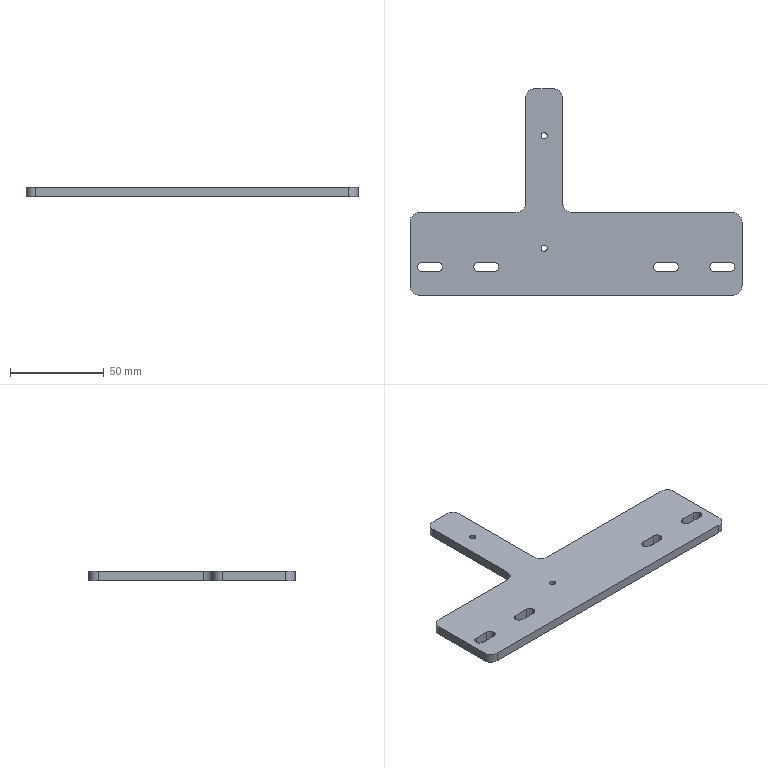Part | 1 solid | 42 faces | box 177 x 110 x 5 mm | volume 44090 mm3 | cylinder 24 | plane 18 | commonest cylinder face diameters 5.2 x12 10 x8 3.3 x4
STEP:
#1=CARTESIAN_POINT('',(-74.3,-40.,0.));
#2=VERTEX_POINT('',#1);
#3=CARTESIAN_POINT('',(-76.9,-37.4,0.));
#4=VERTEX_POINT('',#3);
#5=CARTESIAN_POINT('',(-76.9,-40.,0.));
#6=DIRECTION('',(0.,0.,1.));
#7=DIRECTION('',(1.,0.,0.));
#8=AXIS2_PLACEMENT_3D('',#5,#6,#7);
#9=CIRCLE('',#8,2.6);
#10=EDGE_CURVE('',#2,#4,#9,.T.);
#11=ORIENTED_EDGE('',*,*,#10,.F.);
#12=CARTESIAN_POINT('',(-74.3,-40.,5.));
#13=VERTEX_POINT('',#12);
#14=CARTESIAN_POINT('',(-74.3,-40.,0.));
#15=DIRECTION('',(0.,0.,1.));
#16=VECTOR('',#15,1000.);
#17=LINE('',#14,#16);
#18=EDGE_CURVE('',#2,#13,#17,.T.);
#19=ORIENTED_EDGE('',*,*,#18,.T.);
#20=CARTESIAN_POINT('',(-76.9,-37.4,5.));
#21=VERTEX_POINT('',#20);
#22=CARTESIAN_POINT('',(-76.9,-40.,5.));
#23=DIRECTION('',(0.,0.,1.));
#24=DIRECTION('',(1.,0.,0.));
#25=AXIS2_PLACEMENT_3D('',#22,#23,#24);
#26=CIRCLE('',#25,2.6);
#27=EDGE_CURVE('',#13,#21,#26,.T.);
#28=ORIENTED_EDGE('',*,*,#27,.T.);
#29=CARTESIAN_POINT('',(-76.9,-37.4,0.));
#30=DIRECTION('',(0.,0.,1.));
#31=VECTOR('',#30,1000.);
#32=LINE('',#29,#31);
#33=EDGE_CURVE('',#4,#21,#32,.T.);
#34=ORIENTED_EDGE('',*,*,#33,.F.);
#35=EDGE_LOOP('',(#11,#19,#28,#34));
#36=FACE_OUTER_BOUND('',#35,.T.);
#37=CARTESIAN_POINT('',(-76.9,-40.,0.));
#38=DIRECTION('',(0.,0.,1.));
#39=DIRECTION('',(1.,0.,0.));
#40=AXIS2_PLACEMENT_3D('',#37,#38,#39);
#41=CYLINDRICAL_SURFACE('',#40,2.6);
#42=ADVANCED_FACE('',(#36),#41,.F.);
#43=CARTESIAN_POINT('',(-44.3,-40.,0.));
#44=VERTEX_POINT('',#43);
#45=CARTESIAN_POINT('',(-46.9,-37.4,0.));
#46=VERTEX_POINT('',#45);
#47=CARTESIAN_POINT('',(-46.9,-40.,0.));
#48=DIRECTION('',(0.,0.,1.));
#49=DIRECTION('',(1.,0.,0.));
#50=AXIS2_PLACEMENT_3D('',#47,#48,#49);
#51=CIRCLE('',#50,2.6);
#52=EDGE_CURVE('',#44,#46,#51,.T.);
#53=ORIENTED_EDGE('',*,*,#52,.F.);
#54=CARTESIAN_POINT('',(-44.3,-40.,5.));
#55=VERTEX_POINT('',#54);
#56=CARTESIAN_POINT('',(-44.3,-40.,0.));
#57=DIRECTION('',(0.,0.,1.));
#58=VECTOR('',#57,1000.);
#59=LINE('',#56,#58);
#60=EDGE_CURVE('',#44,#55,#59,.T.);
#61=ORIENTED_EDGE('',*,*,#60,.T.);
#62=CARTESIAN_POINT('',(-46.9,-37.4,5.));
#63=VERTEX_POINT('',#62);
#64=CARTESIAN_POINT('',(-46.9,-40.,5.));
#65=DIRECTION('',(0.,0.,1.));
#66=DIRECTION('',(1.,0.,0.));
#67=AXIS2_PLACEMENT_3D('',#64,#65,#66);
#68=CIRCLE('',#67,2.6);
#69=EDGE_CURVE('',#55,#63,#68,.T.);
#70=ORIENTED_EDGE('',*,*,#69,.T.);
#71=CARTESIAN_POINT('',(-46.9,-37.4,0.));
#72=DIRECTION('',(0.,0.,1.));
#73=VECTOR('',#72,1000.);
#74=LINE('',#71,#73);
#75=EDGE_CURVE('',#46,#63,#74,.T.);
#76=ORIENTED_EDGE('',*,*,#75,.F.);
#77=EDGE_LOOP('',(#53,#61,#70,#76));
#78=FACE_OUTER_BOUND('',#77,.T.);
#79=CARTESIAN_POINT('',(-46.9,-40.,0.));
#80=DIRECTION('',(0.,0.,1.));
#81=DIRECTION('',(1.,0.,0.));
#82=AXIS2_PLACEMENT_3D('',#79,#80,#81);
#83=CYLINDRICAL_SURFACE('',#82,2.6);
#84=ADVANCED_FACE('',(#78),#83,.F.);
#85=CARTESIAN_POINT('',(51.5,-40.,0.));
#86=VERTEX_POINT('',#85);
#87=CARTESIAN_POINT('',(48.9,-37.4,0.));
#88=VERTEX_POINT('',#87);
#89=CARTESIAN_POINT('',(48.9,-40.,0.));
#90=DIRECTION('',(0.,0.,1.));
#91=DIRECTION('',(1.,0.,0.));
#92=AXIS2_PLACEMENT_3D('',#89,#90,#91);
#93=CIRCLE('',#92,2.6);
#94=EDGE_CURVE('',#86,#88,#93,.T.);
#95=ORIENTED_EDGE('',*,*,#94,.F.);
#96=CARTESIAN_POINT('',(51.5,-40.,5.));
#97=VERTEX_POINT('',#96);
#98=CARTESIAN_POINT('',(51.5,-40.,0.));
#99=DIRECTION('',(0.,0.,1.));
#100=VECTOR('',#99,1000.);
#101=LINE('',#98,#100);
#102=EDGE_CURVE('',#86,#97,#101,.T.);
#103=ORIENTED_EDGE('',*,*,#102,.T.);
#104=CARTESIAN_POINT('',(48.9,-37.4,5.));
#105=VERTEX_POINT('',#104);
#106=CARTESIAN_POINT('',(48.9,-40.,5.));
#107=DIRECTION('',(0.,0.,1.));
#108=DIRECTION('',(1.,0.,0.));
#109=AXIS2_PLACEMENT_3D('',#106,#107,#108);
#110=CIRCLE('',#109,2.6);
#111=EDGE_CURVE('',#97,#105,#110,.T.);
#112=ORIENTED_EDGE('',*,*,#111,.T.);
#113=CARTESIAN_POINT('',(48.9,-37.4,0.));
#114=DIRECTION('',(0.,0.,1.));
#115=VECTOR('',#114,1000.);
#116=LINE('',#113,#115);
#117=EDGE_CURVE('',#88,#105,#116,.T.);
#118=ORIENTED_EDGE('',*,*,#117,.F.);
#119=EDGE_LOOP('',(#95,#103,#112,#118));
#120=FACE_OUTER_BOUND('',#119,.T.);
#121=CARTESIAN_POINT('',(48.9,-40.,0.));
#122=DIRECTION('',(0.,0.,1.));
#123=DIRECTION('',(1.,0.,0.));
#124=AXIS2_PLACEMENT_3D('',#121,#122,#123);
#125=CYLINDRICAL_SURFACE('',#124,2.6);
#126=ADVANCED_FACE('',(#120),#125,.F.);
#127=CARTESIAN_POINT('',(81.5,-40.,0.));
#128=VERTEX_POINT('',#127);
#129=CARTESIAN_POINT('',(78.9,-37.4,0.));
#130=VERTEX_POINT('',#129);
#131=CARTESIAN_POINT('',(78.9,-40.,0.));
#132=DIRECTION('',(0.,0.,1.));
#133=DIRECTION('',(1.,0.,0.));
#134=AXIS2_PLACEMENT_3D('',#131,#132,#133);
#135=CIRCLE('',#134,2.6);
#136=EDGE_CURVE('',#128,#130,#135,.T.);
#137=ORIENTED_EDGE('',*,*,#136,.F.);
#138=CARTESIAN_POINT('',(81.5,-40.,5.));
#139=VERTEX_POINT('',#138);
#140=CARTESIAN_POINT('',(81.5,-40.,0.));
#141=DIRECTION('',(0.,0.,1.));
#142=VECTOR('',#141,1000.);
#143=LINE('',#140,#142);
#144=EDGE_CURVE('',#128,#139,#143,.T.);
#145=ORIENTED_EDGE('',*,*,#144,.T.);
#146=CARTESIAN_POINT('',(78.9,-37.4,5.));
#147=VERTEX_POINT('',#146);
#148=CARTESIAN_POINT('',(78.9,-40.,5.));
#149=DIRECTION('',(0.,0.,1.));
#150=DIRECTION('',(1.,0.,0.));
#151=AXIS2_PLACEMENT_3D('',#148,#149,#150);
#152=CIRCLE('',#151,2.6);
#153=EDGE_CURVE('',#139,#147,#152,.T.);
#154=ORIENTED_EDGE('',*,*,#153,.T.);
#155=CARTESIAN_POINT('',(78.9,-37.4,0.));
#156=DIRECTION('',(0.,0.,1.));
#157=VECTOR('',#156,1000.);
#158=LINE('',#155,#157);
#159=EDGE_CURVE('',#130,#147,#158,.T.);
#160=ORIENTED_EDGE('',*,*,#159,.F.);
#161=EDGE_LOOP('',(#137,#145,#154,#160));
#162=FACE_OUTER_BOUND('',#161,.T.);
#163=CARTESIAN_POINT('',(78.9,-40.,0.));
#164=DIRECTION('',(0.,0.,1.));
#165=DIRECTION('',(1.,0.,0.));
#166=AXIS2_PLACEMENT_3D('',#163,#164,#165);
#167=CYLINDRICAL_SURFACE('',#166,2.6);
#168=ADVANCED_FACE('',(#162),#167,.F.);
#169=CARTESIAN_POINT('',(-21.65,30.,0.));
#170=VERTEX_POINT('',#169);
#171=CARTESIAN_POINT('',(-18.35,30.,0.));
#172=VERTEX_POINT('',#171);
#173=CARTESIAN_POINT('',(-20.,30.,0.));
#174=DIRECTION('',(0.,0.,1.));
#175=DIRECTION('',(1.,0.,0.));
#176=AXIS2_PLACEMENT_3D('',#173,#174,#175);
#177=CIRCLE('',#176,1.65);
#178=EDGE_CURVE('',#170,#172,#177,.T.);
#179=ORIENTED_EDGE('',*,*,#178,.F.);
#180=CARTESIAN_POINT('',(-21.65,30.,5.));
#181=VERTEX_POINT('',#180);
#182=CARTESIAN_POINT('',(-21.65,30.,5.));
#183=DIRECTION('',(0.,0.,1.));
#184=VECTOR('',#183,1000.);
#185=LINE('',#182,#184);
#186=EDGE_CURVE('',#170,#181,#185,.T.);
#187=ORIENTED_EDGE('',*,*,#186,.T.);
#188=CARTESIAN_POINT('',(-18.35,30.,5.));
#189=VERTEX_POINT('',#188);
#190=CARTESIAN_POINT('',(-20.,30.,5.));
#191=DIRECTION('',(0.,0.,1.));
#192=DIRECTION('',(1.,0.,0.));
#193=AXIS2_PLACEMENT_3D('',#190,#191,#192);
#194=CIRCLE('',#193,1.65);
#195=EDGE_CURVE('',#181,#189,#194,.T.);
#196=ORIENTED_EDGE('',*,*,#195,.T.);
#197=CARTESIAN_POINT('',(-18.35,30.,5.));
#198=DIRECTION('',(0.,0.,1.));
#199=VECTOR('',#198,1000.);
#200=LINE('',#197,#199);
#201=EDGE_CURVE('',#172,#189,#200,.T.);
#202=ORIENTED_EDGE('',*,*,#201,.F.);
#203=EDGE_LOOP('',(#179,#187,#196,#202));
#204=FACE_OUTER_BOUND('',#203,.T.);
#205=CARTESIAN_POINT('',(-20.,30.,5.));
#206=DIRECTION('',(0.,0.,1.));
#207=DIRECTION('',(1.,0.,0.));
#208=AXIS2_PLACEMENT_3D('',#205,#206,#207);
#209=CYLINDRICAL_SURFACE('',#208,1.65);
#210=ADVANCED_FACE('',(#204),#209,.F.);
#211=CARTESIAN_POINT('',(-21.65,-30.,0.));
#212=VERTEX_POINT('',#211);
#213=CARTESIAN_POINT('',(-18.35,-30.,0.));
#214=VERTEX_POINT('',#213);
#215=CARTESIAN_POINT('',(-20.,-30.,0.));
#216=DIRECTION('',(0.,0.,1.));
#217=DIRECTION('',(1.,0.,0.));
#218=AXIS2_PLACEMENT_3D('',#215,#216,#217);
#219=CIRCLE('',#218,1.65);
#220=EDGE_CURVE('',#212,#214,#219,.T.);
#221=ORIENTED_EDGE('',*,*,#220,.F.);
#222=CARTESIAN_POINT('',(-21.65,-30.,5.));
#223=VERTEX_POINT('',#222);
#224=CARTESIAN_POINT('',(-21.65,-30.,5.));
#225=DIRECTION('',(0.,0.,1.));
#226=VECTOR('',#225,1000.);
#227=LINE('',#224,#226);
#228=EDGE_CURVE('',#212,#223,#227,.T.);
#229=ORIENTED_EDGE('',*,*,#228,.T.);
#230=CARTESIAN_POINT('',(-18.35,-30.,5.));
#231=VERTEX_POINT('',#230);
#232=CARTESIAN_POINT('',(-20.,-30.,5.));
#233=DIRECTION('',(0.,0.,1.));
#234=DIRECTION('',(1.,0.,0.));
#235=AXIS2_PLACEMENT_3D('',#232,#233,#234);
#236=CIRCLE('',#235,1.65);
#237=EDGE_CURVE('',#223,#231,#236,.T.);
#238=ORIENTED_EDGE('',*,*,#237,.T.);
#239=CARTESIAN_POINT('',(-18.35,-30.,5.));
#240=DIRECTION('',(0.,0.,1.));
#241=VECTOR('',#240,1000.);
#242=LINE('',#239,#241);
#243=EDGE_CURVE('',#214,#231,#242,.T.);
#244=ORIENTED_EDGE('',*,*,#243,.F.);
#245=EDGE_LOOP('',(#221,#229,#238,#244));
#246=FACE_OUTER_BOUND('',#245,.T.);
#247=CARTESIAN_POINT('',(-20.,-30.,5.));
#248=DIRECTION('',(0.,0.,1.));
#249=DIRECTION('',(1.,0.,0.));
#250=AXIS2_PLACEMENT_3D('',#247,#248,#249);
#251=CYLINDRICAL_SURFACE('',#250,1.65);
#252=ADVANCED_FACE('',(#246),#251,.F.);
#253=CARTESIAN_POINT('',(-84.9,-37.4,0.));
#254=VERTEX_POINT('',#253);
#255=CARTESIAN_POINT('',(-84.9,-42.6,0.));
#256=VERTEX_POINT('',#255);
#257=CARTESIAN_POINT('',(-84.9,-40.,0.));
#258=DIRECTION('',(0.,0.,1.));
#259=DIRECTION('',(1.,0.,0.));
#260=AXIS2_PLACEMENT_3D('',#257,#258,#259);
#261=CIRCLE('',#260,2.6);
#262=EDGE_CURVE('',#254,#256,#261,.T.);
#263=ORIENTED_EDGE('',*,*,#262,.T.);
#264=CARTESIAN_POINT('',(-76.9,-42.6,0.));
#265=VERTEX_POINT('',#264);
#266=CARTESIAN_POINT('',(-84.9,-42.6,0.));
#267=DIRECTION('',(1.,0.,0.));
#268=VECTOR('',#267,1000.);
#269=LINE('',#266,#268);
#270=EDGE_CURVE('',#256,#265,#269,.T.);
#271=ORIENTED_EDGE('',*,*,#270,.T.);
#272=CARTESIAN_POINT('',(-76.9,-40.,0.));
#273=DIRECTION('',(0.,0.,1.));
#274=DIRECTION('',(1.,0.,0.));
#275=AXIS2_PLACEMENT_3D('',#272,#273,#274);
#276=CIRCLE('',#275,2.6);
#277=EDGE_CURVE('',#265,#2,#276,.T.);
#278=ORIENTED_EDGE('',*,*,#277,.T.);
#279=ORIENTED_EDGE('',*,*,#10,.T.);
#280=CARTESIAN_POINT('',(-84.9,-37.4,0.));
#281=DIRECTION('',(-1.,0.,0.));
#282=VECTOR('',#281,1000.);
#283=LINE('',#280,#282);
#284=EDGE_CURVE('',#4,#254,#283,.T.);
#285=ORIENTED_EDGE('',*,*,#284,.T.);
#286=EDGE_LOOP('',(#263,#271,#278,#279,#285));
#287=FACE_BOUND('',#286,.T.);
#288=CARTESIAN_POINT('',(-54.9,-37.4,0.));
#289=VERTEX_POINT('',#288);
#290=CARTESIAN_POINT('',(-54.9,-42.6,0.));
#291=VERTEX_POINT('',#290);
#292=CARTESIAN_POINT('',(-54.9,-40.,0.));
#293=DIRECTION('',(0.,0.,1.));
#294=DIRECTION('',(1.,0.,0.));
#295=AXIS2_PLACEMENT_3D('',#292,#293,#294);
#296=CIRCLE('',#295,2.6);
#297=EDGE_CURVE('',#289,#291,#296,.T.);
#298=ORIENTED_EDGE('',*,*,#297,.T.);
#299=CARTESIAN_POINT('',(-46.9,-42.6,0.));
#300=VERTEX_POINT('',#299);
#301=CARTESIAN_POINT('',(-54.9,-42.6,0.));
#302=DIRECTION('',(1.,0.,0.));
#303=VECTOR('',#302,1000.);
#304=LINE('',#301,#303);
#305=EDGE_CURVE('',#291,#300,#304,.T.);
#306=ORIENTED_EDGE('',*,*,#305,.T.);
#307=CARTESIAN_POINT('',(-46.9,-40.,0.));
#308=DIRECTION('',(0.,0.,1.));
#309=DIRECTION('',(1.,0.,0.));
#310=AXIS2_PLACEMENT_3D('',#307,#308,#309);
#311=CIRCLE('',#310,2.6);
#312=EDGE_CURVE('',#300,#44,#311,.T.);
#313=ORIENTED_EDGE('',*,*,#312,.T.);
#314=ORIENTED_EDGE('',*,*,#52,.T.);
#315=CARTESIAN_POINT('',(-54.9,-37.4,0.));
#316=DIRECTION('',(-1.,0.,0.));
#317=VECTOR('',#316,1000.);
#318=LINE('',#315,#317);
#319=EDGE_CURVE('',#46,#289,#318,.T.);
#320=ORIENTED_EDGE('',*,*,#319,.T.);
#321=EDGE_LOOP('',(#298,#306,#313,#314,#320));
#322=FACE_BOUND('',#321,.T.);
#323=CARTESIAN_POINT('',(40.9,-37.4,0.));
#324=VERTEX_POINT('',#323);
#325=CARTESIAN_POINT('',(40.9,-42.6,0.));
#326=VERTEX_POINT('',#325);
#327=CARTESIAN_POINT('',(40.9,-40.,0.));
#328=DIRECTION('',(0.,0.,1.));
#329=DIRECTION('',(1.,0.,0.));
#330=AXIS2_PLACEMENT_3D('',#327,#328,#329);
#331=CIRCLE('',#330,2.6);
#332=EDGE_CURVE('',#324,#326,#331,.T.);
#333=ORIENTED_EDGE('',*,*,#332,.T.);
#334=CARTESIAN_POINT('',(48.9,-42.6,0.));
#335=VERTEX_POINT('',#334);
#336=CARTESIAN_POINT('',(40.9,-42.6,0.));
#337=DIRECTION('',(1.,0.,0.));
#338=VECTOR('',#337,1000.);
#339=LINE('',#336,#338);
#340=EDGE_CURVE('',#326,#335,#339,.T.);
#341=ORIENTED_EDGE('',*,*,#340,.T.);
#342=CARTESIAN_POINT('',(48.9,-40.,0.));
#343=DIRECTION('',(0.,0.,1.));
#344=DIRECTION('',(1.,0.,0.));
#345=AXIS2_PLACEMENT_3D('',#342,#343,#344);
#346=CIRCLE('',#345,2.6);
#347=EDGE_CURVE('',#335,#86,#346,.T.);
#348=ORIENTED_EDGE('',*,*,#347,.T.);
#349=ORIENTED_EDGE('',*,*,#94,.T.);
#350=CARTESIAN_POINT('',(40.9,-37.4,0.));
#351=DIRECTION('',(-1.,0.,0.));
#352=VECTOR('',#351,1000.);
#353=LINE('',#350,#352);
#354=EDGE_CURVE('',#88,#324,#353,.T.);
#355=ORIENTED_EDGE('',*,*,#354,.T.);
#356=EDGE_LOOP('',(#333,#341,#348,#349,#355));
#357=FACE_BOUND('',#356,.T.);
#358=CARTESIAN_POINT('',(70.9,-37.4,0.));
#359=VERTEX_POINT('',#358);
#360=CARTESIAN_POINT('',(70.9,-42.6,0.));
#361=VERTEX_POINT('',#360);
#362=CARTESIAN_POINT('',(70.9,-40.,0.));
#363=DIRECTION('',(0.,0.,1.));
#364=DIRECTION('',(1.,0.,0.));
#365=AXIS2_PLACEMENT_3D('',#362,#363,#364);
#366=CIRCLE('',#365,2.6);
#367=EDGE_CURVE('',#359,#361,#366,.T.);
#368=ORIENTED_EDGE('',*,*,#367,.T.);
#369=CARTESIAN_POINT('',(78.9,-42.6,0.));
#370=VERTEX_POINT('',#369);
#371=CARTESIAN_POINT('',(70.9,-42.6,0.));
#372=DIRECTION('',(1.,0.,0.));
#373=VECTOR('',#372,1000.);
#374=LINE('',#371,#373);
#375=EDGE_CURVE('',#361,#370,#374,.T.);
#376=ORIENTED_EDGE('',*,*,#375,.T.);
#377=CARTESIAN_POINT('',(78.9,-40.,0.));
#378=DIRECTION('',(0.,0.,1.));
#379=DIRECTION('',(1.,0.,0.));
#380=AXIS2_PLACEMENT_3D('',#377,#378,#379);
#381=CIRCLE('',#380,2.6);
#382=EDGE_CURVE('',#370,#128,#381,.T.);
#383=ORIENTED_EDGE('',*,*,#382,.T.);
#384=ORIENTED_EDGE('',*,*,#136,.T.);
#385=CARTESIAN_POINT('',(70.9,-37.4,0.));
#386=DIRECTION('',(-1.,0.,0.));
#387=VECTOR('',#386,1000.);
#388=LINE('',#385,#387);
#389=EDGE_CURVE('',#130,#359,#388,.T.);
#390=ORIENTED_EDGE('',*,*,#389,.T.);
#391=EDGE_LOOP('',(#368,#376,#383,#384,#390));
#392=FACE_BOUND('',#391,.T.);
#393=CARTESIAN_POINT('',(-86.5,-55.,0.));
#394=VERTEX_POINT('',#393);
#395=CARTESIAN_POINT('',(80.5,-55.,0.));
#396=VERTEX_POINT('',#395);
#397=CARTESIAN_POINT('',(-88.5,-55.,0.));
#398=DIRECTION('',(1.,0.,0.));
#399=VECTOR('',#398,1000.);
#400=LINE('',#397,#399);
#401=EDGE_CURVE('',#394,#396,#400,.T.);
#402=ORIENTED_EDGE('',*,*,#401,.F.);
#403=CARTESIAN_POINT('',(-91.5,-50.,0.));
#404=VERTEX_POINT('',#403);
#405=CARTESIAN_POINT('',(-86.5,-50.,0.));
#406=DIRECTION('',(0.,0.,-1.));
#407=DIRECTION('',(-1.,0.,0.));
#408=AXIS2_PLACEMENT_3D('',#405,#406,#407);
#409=CIRCLE('',#408,5.);
#410=EDGE_CURVE('',#394,#404,#409,.T.);
#411=ORIENTED_EDGE('',*,*,#410,.T.);
#412=CARTESIAN_POINT('',(-91.5,-16.,0.));
#413=VERTEX_POINT('',#412);
#414=CARTESIAN_POINT('',(-91.5,-55.,0.));
#415=DIRECTION('',(0.,-1.,0.));
#416=VECTOR('',#415,1000.);
#417=LINE('',#414,#416);
#418=EDGE_CURVE('',#413,#404,#417,.T.);
#419=ORIENTED_EDGE('',*,*,#418,.F.);
#420=CARTESIAN_POINT('',(-86.5,-11.,0.));
#421=VERTEX_POINT('',#420);
#422=CARTESIAN_POINT('',(-86.5,-16.,0.));
#423=DIRECTION('',(0.,0.,-1.));
#424=DIRECTION('',(-1.,0.,0.));
#425=AXIS2_PLACEMENT_3D('',#422,#423,#424);
#426=CIRCLE('',#425,5.);
#427=EDGE_CURVE('',#413,#421,#426,.T.);
#428=ORIENTED_EDGE('',*,*,#427,.T.);
#429=CARTESIAN_POINT('',(-35.,-11.,0.));
#430=VERTEX_POINT('',#429);
#431=CARTESIAN_POINT('',(0.,-11.,0.));
#432=DIRECTION('',(-1.,0.,0.));
#433=VECTOR('',#432,1000.);
#434=LINE('',#431,#433);
#435=EDGE_CURVE('',#430,#421,#434,.T.);
#436=ORIENTED_EDGE('',*,*,#435,.F.);
#437=CARTESIAN_POINT('',(-30.,-6.,0.));
#438=VERTEX_POINT('',#437);
#439=CARTESIAN_POINT('',(-35.,-6.,0.));
#440=DIRECTION('',(0.,0.,1.));
#441=DIRECTION('',(-1.,0.,0.));
#442=AXIS2_PLACEMENT_3D('',#439,#440,#441);
#443=CIRCLE('',#442,5.);
#444=EDGE_CURVE('',#430,#438,#443,.T.);
#445=ORIENTED_EDGE('',*,*,#444,.T.);
#446=CARTESIAN_POINT('',(-30.,50.,0.));
#447=VERTEX_POINT('',#446);
#448=CARTESIAN_POINT('',(-30.,0.,0.));
#449=DIRECTION('',(0.,-1.,0.));
#450=VECTOR('',#449,1000.);
#451=LINE('',#448,#450);
#452=EDGE_CURVE('',#447,#438,#451,.T.);
#453=ORIENTED_EDGE('',*,*,#452,.F.);
#454=CARTESIAN_POINT('',(-25.,55.,0.));
#455=VERTEX_POINT('',#454);
#456=CARTESIAN_POINT('',(-25.,50.,0.));
#457=DIRECTION('',(0.,0.,-1.));
#458=DIRECTION('',(-1.,0.,0.));
#459=AXIS2_PLACEMENT_3D('',#456,#457,#458);
#460=CIRCLE('',#459,5.);
#461=EDGE_CURVE('',#447,#455,#460,.T.);
#462=ORIENTED_EDGE('',*,*,#461,.T.);
#463=CARTESIAN_POINT('',(-15.,55.,0.));
#464=VERTEX_POINT('',#463);
#465=CARTESIAN_POINT('',(-88.5,55.,0.));
#466=DIRECTION('',(-1.,0.,0.));
#467=VECTOR('',#466,1000.);
#468=LINE('',#465,#467);
#469=EDGE_CURVE('',#464,#455,#468,.T.);
#470=ORIENTED_EDGE('',*,*,#469,.F.);
#471=CARTESIAN_POINT('',(-10.,50.,0.));
#472=VERTEX_POINT('',#471);
#473=CARTESIAN_POINT('',(-15.,50.,0.));
#474=DIRECTION('',(0.,0.,-1.));
#475=DIRECTION('',(-1.,0.,0.));
#476=AXIS2_PLACEMENT_3D('',#473,#474,#475);
#477=CIRCLE('',#476,5.);
#478=EDGE_CURVE('',#464,#472,#477,.T.);
#479=ORIENTED_EDGE('',*,*,#478,.T.);
#480=CARTESIAN_POINT('',(-10.,-6.,0.));
#481=VERTEX_POINT('',#480);
#482=CARTESIAN_POINT('',(-10.,55.,0.));
#483=DIRECTION('',(0.,-1.,0.));
#484=VECTOR('',#483,1000.);
#485=LINE('',#482,#484);
#486=EDGE_CURVE('',#472,#481,#485,.T.);
#487=ORIENTED_EDGE('',*,*,#486,.T.);
#488=CARTESIAN_POINT('',(-5.,-11.,0.));
#489=VERTEX_POINT('',#488);
#490=CARTESIAN_POINT('',(-5.,-6.,0.));
#491=DIRECTION('',(0.,0.,1.));
#492=DIRECTION('',(-1.,0.,0.));
#493=AXIS2_PLACEMENT_3D('',#490,#491,#492);
#494=CIRCLE('',#493,5.);
#495=EDGE_CURVE('',#481,#489,#494,.T.);
#496=ORIENTED_EDGE('',*,*,#495,.T.);
#497=CARTESIAN_POINT('',(80.5,-11.,0.));
#498=VERTEX_POINT('',#497);
#499=CARTESIAN_POINT('',(-10.,-11.,0.));
#500=DIRECTION('',(1.,0.,0.));
#501=VECTOR('',#500,1000.);
#502=LINE('',#499,#501);
#503=EDGE_CURVE('',#489,#498,#502,.T.);
#504=ORIENTED_EDGE('',*,*,#503,.T.);
#505=CARTESIAN_POINT('',(85.5,-16.,0.));
#506=VERTEX_POINT('',#505);
#507=CARTESIAN_POINT('',(80.5,-16.,0.));
#508=DIRECTION('',(0.,0.,-1.));
#509=DIRECTION('',(-1.,0.,0.));
#510=AXIS2_PLACEMENT_3D('',#507,#508,#509);
#511=CIRCLE('',#510,5.);
#512=EDGE_CURVE('',#498,#506,#511,.T.);
#513=ORIENTED_EDGE('',*,*,#512,.T.);
#514=CARTESIAN_POINT('',(85.5,-50.,0.));
#515=VERTEX_POINT('',#514);
#516=CARTESIAN_POINT('',(85.5,-55.,0.));
#517=DIRECTION('',(0.,1.,0.));
#518=VECTOR('',#517,1000.);
#519=LINE('',#516,#518);
#520=EDGE_CURVE('',#515,#506,#519,.T.);
#521=ORIENTED_EDGE('',*,*,#520,.F.);
#522=CARTESIAN_POINT('',(80.5,-50.,0.));
#523=DIRECTION('',(0.,0.,-1.));
#524=DIRECTION('',(-1.,0.,0.));
#525=AXIS2_PLACEMENT_3D('',#522,#523,#524);
#526=CIRCLE('',#525,5.);
#527=EDGE_CURVE('',#515,#396,#526,.T.);
#528=ORIENTED_EDGE('',*,*,#527,.T.);
#529=EDGE_LOOP('',(#402,#411,#419,#428,#436,#445,#453,#462,#470,#479,#487,#496,#504,#513,#521,#528));
#530=FACE_OUTER_BOUND('',#529,.T.);
#531=CARTESIAN_POINT('',(-20.,30.,0.));
#532=DIRECTION('',(0.,0.,1.));
#533=DIRECTION('',(1.,0.,0.));
#534=AXIS2_PLACEMENT_3D('',#531,#532,#533);
#535=CIRCLE('',#534,1.65);
#536=EDGE_CURVE('',#172,#170,#535,.T.);
#537=ORIENTED_EDGE('',*,*,#536,.T.);
#538=ORIENTED_EDGE('',*,*,#178,.T.);
#539=EDGE_LOOP('',(#537,#538));
#540=FACE_BOUND('',#539,.T.);
#541=CARTESIAN_POINT('',(-20.,-30.,0.));
#542=DIRECTION('',(0.,0.,1.));
#543=DIRECTION('',(1.,0.,0.));
#544=AXIS2_PLACEMENT_3D('',#541,#542,#543);
#545=CIRCLE('',#544,1.65);
#546=EDGE_CURVE('',#214,#212,#545,.T.);
#547=ORIENTED_EDGE('',*,*,#546,.T.);
#548=ORIENTED_EDGE('',*,*,#220,.T.);
#549=EDGE_LOOP('',(#547,#548));
#550=FACE_BOUND('',#549,.T.);
#551=CARTESIAN_POINT('',(0.,0.,0.));
#552=DIRECTION('',(0.,0.,-1.));
#553=DIRECTION('',(-1.,0.,0.));
#554=AXIS2_PLACEMENT_3D('',#551,#552,#553);
#555=PLANE('',#554);
#556=ADVANCED_FACE('',(#287,#322,#357,#392,#530,#540,#550),#555,.T.);
#557=CARTESIAN_POINT('',(85.5,-50.,5.));
#558=VERTEX_POINT('',#557);
#559=CARTESIAN_POINT('',(85.5,-16.,5.));
#560=VERTEX_POINT('',#559);
#561=CARTESIAN_POINT('',(85.5,-55.,5.));
#562=DIRECTION('',(0.,1.,0.));
#563=VECTOR('',#562,1000.);
#564=LINE('',#561,#563);
#565=EDGE_CURVE('',#558,#560,#564,.T.);
#566=ORIENTED_EDGE('',*,*,#565,.F.);
#567=CARTESIAN_POINT('',(85.5,-50.,5.));
#568=DIRECTION('',(0.,0.,-1.));
#569=VECTOR('',#568,1000.);
#570=LINE('',#567,#569);
#571=EDGE_CURVE('',#558,#515,#570,.T.);
#572=ORIENTED_EDGE('',*,*,#571,.T.);
#573=ORIENTED_EDGE('',*,*,#520,.T.);
#574=CARTESIAN_POINT('',(85.5,-16.,5.));
#575=DIRECTION('',(0.,0.,1.));
#576=VECTOR('',#575,1000.);
#577=LINE('',#574,#576);
#578=EDGE_CURVE('',#506,#560,#577,.T.);
#579=ORIENTED_EDGE('',*,*,#578,.T.);
#580=EDGE_LOOP('',(#566,#572,#573,#579));
#581=FACE_OUTER_BOUND('',#580,.T.);
#582=CARTESIAN_POINT('',(85.5,-55.,5.));
#583=DIRECTION('',(-1.,0.,0.));
#584=DIRECTION('',(0.,-1.,0.));
#585=AXIS2_PLACEMENT_3D('',#582,#583,#584);
#586=PLANE('',#585);
#587=ADVANCED_FACE('',(#581),#586,.F.);
#588=CARTESIAN_POINT('',(-15.,55.,5.));
#589=VERTEX_POINT('',#588);
#590=CARTESIAN_POINT('',(-25.,55.,5.));
#591=VERTEX_POINT('',#590);
#592=CARTESIAN_POINT('',(-88.5,55.,5.));
#593=DIRECTION('',(-1.,0.,0.));
#594=VECTOR('',#593,1000.);
#595=LINE('',#592,#594);
#596=EDGE_CURVE('',#589,#591,#595,.T.);
#597=ORIENTED_EDGE('',*,*,#596,.F.);
#598=CARTESIAN_POINT('',(-15.,55.,5.));
#599=DIRECTION('',(0.,0.,-1.));
#600=VECTOR('',#599,1000.);
#601=LINE('',#598,#600);
#602=EDGE_CURVE('',#589,#464,#601,.T.);
#603=ORIENTED_EDGE('',*,*,#602,.T.);
#604=ORIENTED_EDGE('',*,*,#469,.T.);
#605=CARTESIAN_POINT('',(-25.,55.,5.));
#606=DIRECTION('',(0.,0.,1.));
#607=VECTOR('',#606,1000.);
#608=LINE('',#605,#607);
#609=EDGE_CURVE('',#455,#591,#608,.T.);
#610=ORIENTED_EDGE('',*,*,#609,.T.);
#611=EDGE_LOOP('',(#597,#603,#604,#610));
#612=FACE_OUTER_BOUND('',#611,.T.);
#613=CARTESIAN_POINT('',(-88.5,55.,5.));
#614=DIRECTION('',(0.,-1.,0.));
#615=DIRECTION('',(1.,0.,0.));
#616=AXIS2_PLACEMENT_3D('',#613,#614,#615);
#617=PLANE('',#616);
#618=ADVANCED_FACE('',(#612),#617,.F.);
#619=ORIENTED_EDGE('',*,*,#418,.T.);
#620=CARTESIAN_POINT('',(-91.5,-50.,5.));
#621=VERTEX_POINT('',#620);
#622=CARTESIAN_POINT('',(-91.5,-50.,5.));
#623=DIRECTION('',(0.,0.,1.));
#624=VECTOR('',#623,1000.);
#625=LINE('',#622,#624);
#626=EDGE_CURVE('',#404,#621,#625,.T.);
#627=ORIENTED_EDGE('',*,*,#626,.T.);
#628=CARTESIAN_POINT('',(-91.5,-16.,5.));
#629=VERTEX_POINT('',#628);
#630=CARTESIAN_POINT('',(-91.5,-55.,5.));
#631=DIRECTION('',(0.,-1.,0.));
#632=VECTOR('',#631,1000.);
#633=LINE('',#630,#632);
#634=EDGE_CURVE('',#629,#621,#633,.T.);
#635=ORIENTED_EDGE('',*,*,#634,.F.);
#636=CARTESIAN_POINT('',(-91.5,-16.,5.));
#637=DIRECTION('',(0.,0.,-1.));
#638=VECTOR('',#637,1000.);
#639=LINE('',#636,#638);
#640=EDGE_CURVE('',#629,#413,#639,.T.);
#641=ORIENTED_EDGE('',*,*,#640,.T.);
#642=EDGE_LOOP('',(#619,#627,#635,#641));
#643=FACE_OUTER_BOUND('',#642,.T.);
#644=CARTESIAN_POINT('',(-91.5,-55.,5.));
#645=DIRECTION('',(1.,0.,0.));
#646=DIRECTION('',(0.,1.,0.));
#647=AXIS2_PLACEMENT_3D('',#644,#645,#646);
#648=PLANE('',#647);
#649=ADVANCED_FACE('',(#643),#648,.F.);
#650=CARTESIAN_POINT('',(-86.5,-55.,5.));
#651=VERTEX_POINT('',#650);
#652=CARTESIAN_POINT('',(80.5,-55.,5.));
#653=VERTEX_POINT('',#652);
#654=CARTESIAN_POINT('',(-88.5,-55.,5.));
#655=DIRECTION('',(1.,0.,0.));
#656=VECTOR('',#655,1000.);
#657=LINE('',#654,#656);
#658=EDGE_CURVE('',#651,#653,#657,.T.);
#659=ORIENTED_EDGE('',*,*,#658,.F.);
#660=CARTESIAN_POINT('',(-86.5,-55.,5.));
#661=DIRECTION('',(0.,0.,-1.));
#662=VECTOR('',#661,1000.);
#663=LINE('',#660,#662);
#664=EDGE_CURVE('',#651,#394,#663,.T.);
#665=ORIENTED_EDGE('',*,*,#664,.T.);
#666=ORIENTED_EDGE('',*,*,#401,.T.);
#667=CARTESIAN_POINT('',(80.5,-55.,5.));
#668=DIRECTION('',(0.,0.,1.));
#669=VECTOR('',#668,1000.);
#670=LINE('',#667,#669);
#671=EDGE_CURVE('',#396,#653,#670,.T.);
#672=ORIENTED_EDGE('',*,*,#671,.T.);
#673=EDGE_LOOP('',(#659,#665,#666,#672));
#674=FACE_OUTER_BOUND('',#673,.T.);
#675=CARTESIAN_POINT('',(-88.5,-55.,5.));
#676=DIRECTION('',(0.,1.,0.));
#677=DIRECTION('',(-1.,0.,0.));
#678=AXIS2_PLACEMENT_3D('',#675,#676,#677);
#679=PLANE('',#678);
#680=ADVANCED_FACE('',(#674),#679,.F.);
#681=CARTESIAN_POINT('',(-84.9,-42.6,5.));
#682=VERTEX_POINT('',#681);
#683=CARTESIAN_POINT('',(-76.9,-42.6,5.));
#684=VERTEX_POINT('',#683);
#685=CARTESIAN_POINT('',(-84.9,-42.6,5.));
#686=DIRECTION('',(1.,0.,0.));
#687=VECTOR('',#686,1000.);
#688=LINE('',#685,#687);
#689=EDGE_CURVE('',#682,#684,#688,.T.);
#690=ORIENTED_EDGE('',*,*,#689,.F.);
#691=CARTESIAN_POINT('',(-84.9,-37.4,5.));
#692=VERTEX_POINT('',#691);
#693=CARTESIAN_POINT('',(-84.9,-40.,5.));
#694=DIRECTION('',(0.,0.,1.));
#695=DIRECTION('',(1.,0.,0.));
#696=AXIS2_PLACEMENT_3D('',#693,#694,#695);
#697=CIRCLE('',#696,2.6);
#698=EDGE_CURVE('',#692,#682,#697,.T.);
#699=ORIENTED_EDGE('',*,*,#698,.F.);
#700=CARTESIAN_POINT('',(-84.9,-37.4,5.));
#701=DIRECTION('',(-1.,0.,0.));
#702=VECTOR('',#701,1000.);
#703=LINE('',#700,#702);
#704=EDGE_CURVE('',#21,#692,#703,.T.);
#705=ORIENTED_EDGE('',*,*,#704,.F.);
#706=ORIENTED_EDGE('',*,*,#27,.F.);
#707=CARTESIAN_POINT('',(-76.9,-40.,5.));
#708=DIRECTION('',(0.,0.,1.));
#709=DIRECTION('',(1.,0.,0.));
#710=AXIS2_PLACEMENT_3D('',#707,#708,#709);
#711=CIRCLE('',#710,2.6);
#712=EDGE_CURVE('',#684,#13,#711,.T.);
#713=ORIENTED_EDGE('',*,*,#712,.F.);
#714=EDGE_LOOP('',(#690,#699,#705,#706,#713));
#715=FACE_BOUND('',#714,.T.);
#716=CARTESIAN_POINT('',(-54.9,-42.6,5.));
#717=VERTEX_POINT('',#716);
#718=CARTESIAN_POINT('',(-46.9,-42.6,5.));
#719=VERTEX_POINT('',#718);
#720=CARTESIAN_POINT('',(-54.9,-42.6,5.));
#721=DIRECTION('',(1.,0.,0.));
#722=VECTOR('',#721,1000.);
#723=LINE('',#720,#722);
#724=EDGE_CURVE('',#717,#719,#723,.T.);
#725=ORIENTED_EDGE('',*,*,#724,.F.);
#726=CARTESIAN_POINT('',(-54.9,-37.4,5.));
#727=VERTEX_POINT('',#726);
#728=CARTESIAN_POINT('',(-54.9,-40.,5.));
#729=DIRECTION('',(0.,0.,1.));
#730=DIRECTION('',(1.,0.,0.));
#731=AXIS2_PLACEMENT_3D('',#728,#729,#730);
#732=CIRCLE('',#731,2.6);
#733=EDGE_CURVE('',#727,#717,#732,.T.);
#734=ORIENTED_EDGE('',*,*,#733,.F.);
#735=CARTESIAN_POINT('',(-54.9,-37.4,5.));
#736=DIRECTION('',(-1.,0.,0.));
#737=VECTOR('',#736,1000.);
#738=LINE('',#735,#737);
#739=EDGE_CURVE('',#63,#727,#738,.T.);
#740=ORIENTED_EDGE('',*,*,#739,.F.);
#741=ORIENTED_EDGE('',*,*,#69,.F.);
#742=CARTESIAN_POINT('',(-46.9,-40.,5.));
#743=DIRECTION('',(0.,0.,1.));
#744=DIRECTION('',(1.,0.,0.));
#745=AXIS2_PLACEMENT_3D('',#742,#743,#744);
#746=CIRCLE('',#745,2.6);
#747=EDGE_CURVE('',#719,#55,#746,.T.);
#748=ORIENTED_EDGE('',*,*,#747,.F.);
#749=EDGE_LOOP('',(#725,#734,#740,#741,#748));
#750=FACE_BOUND('',#749,.T.);
#751=CARTESIAN_POINT('',(40.9,-42.6,5.));
#752=VERTEX_POINT('',#751);
#753=CARTESIAN_POINT('',(48.9,-42.6,5.));
#754=VERTEX_POINT('',#753);
#755=CARTESIAN_POINT('',(40.9,-42.6,5.));
#756=DIRECTION('',(1.,0.,0.));
#757=VECTOR('',#756,1000.);
#758=LINE('',#755,#757);
#759=EDGE_CURVE('',#752,#754,#758,.T.);
#760=ORIENTED_EDGE('',*,*,#759,.F.);
#761=CARTESIAN_POINT('',(40.9,-37.4,5.));
#762=VERTEX_POINT('',#761);
#763=CARTESIAN_POINT('',(40.9,-40.,5.));
#764=DIRECTION('',(0.,0.,1.));
#765=DIRECTION('',(1.,0.,0.));
#766=AXIS2_PLACEMENT_3D('',#763,#764,#765);
#767=CIRCLE('',#766,2.6);
#768=EDGE_CURVE('',#762,#752,#767,.T.);
#769=ORIENTED_EDGE('',*,*,#768,.F.);
#770=CARTESIAN_POINT('',(40.9,-37.4,5.));
#771=DIRECTION('',(-1.,0.,0.));
#772=VECTOR('',#771,1000.);
#773=LINE('',#770,#772);
#774=EDGE_CURVE('',#105,#762,#773,.T.);
#775=ORIENTED_EDGE('',*,*,#774,.F.);
#776=ORIENTED_EDGE('',*,*,#111,.F.);
#777=CARTESIAN_POINT('',(48.9,-40.,5.));
#778=DIRECTION('',(0.,0.,1.));
#779=DIRECTION('',(1.,0.,0.));
#780=AXIS2_PLACEMENT_3D('',#777,#778,#779);
#781=CIRCLE('',#780,2.6);
#782=EDGE_CURVE('',#754,#97,#781,.T.);
#783=ORIENTED_EDGE('',*,*,#782,.F.);
#784=EDGE_LOOP('',(#760,#769,#775,#776,#783));
#785=FACE_BOUND('',#784,.T.);
#786=CARTESIAN_POINT('',(70.9,-42.6,5.));
#787=VERTEX_POINT('',#786);
#788=CARTESIAN_POINT('',(78.9,-42.6,5.));
#789=VERTEX_POINT('',#788);
#790=CARTESIAN_POINT('',(70.9,-42.6,5.));
#791=DIRECTION('',(1.,0.,0.));
#792=VECTOR('',#791,1000.);
#793=LINE('',#790,#792);
#794=EDGE_CURVE('',#787,#789,#793,.T.);
#795=ORIENTED_EDGE('',*,*,#794,.F.);
#796=CARTESIAN_POINT('',(70.9,-37.4,5.));
#797=VERTEX_POINT('',#796);
#798=CARTESIAN_POINT('',(70.9,-40.,5.));
#799=DIRECTION('',(0.,0.,1.));
#800=DIRECTION('',(1.,0.,0.));
#801=AXIS2_PLACEMENT_3D('',#798,#799,#800);
#802=CIRCLE('',#801,2.6);
#803=EDGE_CURVE('',#797,#787,#802,.T.);
#804=ORIENTED_EDGE('',*,*,#803,.F.);
#805=CARTESIAN_POINT('',(70.9,-37.4,5.));
#806=DIRECTION('',(-1.,0.,0.));
#807=VECTOR('',#806,1000.);
#808=LINE('',#805,#807);
#809=EDGE_CURVE('',#147,#797,#808,.T.);
#810=ORIENTED_EDGE('',*,*,#809,.F.);
#811=ORIENTED_EDGE('',*,*,#153,.F.);
#812=CARTESIAN_POINT('',(78.9,-40.,5.));
#813=DIRECTION('',(0.,0.,1.));
#814=DIRECTION('',(1.,0.,0.));
#815=AXIS2_PLACEMENT_3D('',#812,#813,#814);
#816=CIRCLE('',#815,2.6);
#817=EDGE_CURVE('',#789,#139,#816,.T.);
#818=ORIENTED_EDGE('',*,*,#817,.F.);
#819=EDGE_LOOP('',(#795,#804,#810,#811,#818));
#820=FACE_BOUND('',#819,.T.);
#821=CARTESIAN_POINT('',(-20.,30.,5.));
#822=DIRECTION('',(0.,0.,1.));
#823=DIRECTION('',(1.,0.,0.));
#824=AXIS2_PLACEMENT_3D('',#821,#822,#823);
#825=CIRCLE('',#824,1.65);
#826=EDGE_CURVE('',#189,#181,#825,.T.);
#827=ORIENTED_EDGE('',*,*,#826,.F.);
#828=ORIENTED_EDGE('',*,*,#195,.F.);
#829=EDGE_LOOP('',(#827,#828));
#830=FACE_BOUND('',#829,.T.);
#831=CARTESIAN_POINT('',(-20.,-30.,5.));
#832=DIRECTION('',(0.,0.,1.));
#833=DIRECTION('',(1.,0.,0.));
#834=AXIS2_PLACEMENT_3D('',#831,#832,#833);
#835=CIRCLE('',#834,1.65);
#836=EDGE_CURVE('',#231,#223,#835,.T.);
#837=ORIENTED_EDGE('',*,*,#836,.F.);
#838=ORIENTED_EDGE('',*,*,#237,.F.);
#839=EDGE_LOOP('',(#837,#838));
#840=FACE_BOUND('',#839,.T.);
#841=ORIENTED_EDGE('',*,*,#634,.T.);
#842=CARTESIAN_POINT('',(-86.5,-50.,5.));
#843=DIRECTION('',(0.,0.,1.));
#844=DIRECTION('',(-1.,0.,0.));
#845=AXIS2_PLACEMENT_3D('',#842,#843,#844);
#846=CIRCLE('',#845,5.);
#847=EDGE_CURVE('',#621,#651,#846,.T.);
#848=ORIENTED_EDGE('',*,*,#847,.T.);
#849=ORIENTED_EDGE('',*,*,#658,.T.);
#850=CARTESIAN_POINT('',(80.5,-50.,5.));
#851=DIRECTION('',(0.,0.,1.));
#852=DIRECTION('',(-1.,0.,0.));
#853=AXIS2_PLACEMENT_3D('',#850,#851,#852);
#854=CIRCLE('',#853,5.);
#855=EDGE_CURVE('',#653,#558,#854,.T.);
#856=ORIENTED_EDGE('',*,*,#855,.T.);
#857=ORIENTED_EDGE('',*,*,#565,.T.);
#858=CARTESIAN_POINT('',(80.5,-11.,5.));
#859=VERTEX_POINT('',#858);
#860=CARTESIAN_POINT('',(80.5,-16.,5.));
#861=DIRECTION('',(0.,0.,1.));
#862=DIRECTION('',(-1.,0.,0.));
#863=AXIS2_PLACEMENT_3D('',#860,#861,#862);
#864=CIRCLE('',#863,5.);
#865=EDGE_CURVE('',#560,#859,#864,.T.);
#866=ORIENTED_EDGE('',*,*,#865,.T.);
#867=CARTESIAN_POINT('',(-5.,-11.,5.));
#868=VERTEX_POINT('',#867);
#869=CARTESIAN_POINT('',(-10.,-11.,5.));
#870=DIRECTION('',(1.,0.,0.));
#871=VECTOR('',#870,1000.);
#872=LINE('',#869,#871);
#873=EDGE_CURVE('',#868,#859,#872,.T.);
#874=ORIENTED_EDGE('',*,*,#873,.F.);
#875=CARTESIAN_POINT('',(-10.,-6.,5.));
#876=VERTEX_POINT('',#875);
#877=CARTESIAN_POINT('',(-5.,-6.,5.));
#878=DIRECTION('',(0.,0.,-1.));
#879=DIRECTION('',(-1.,0.,0.));
#880=AXIS2_PLACEMENT_3D('',#877,#878,#879);
#881=CIRCLE('',#880,5.);
#882=EDGE_CURVE('',#868,#876,#881,.T.);
#883=ORIENTED_EDGE('',*,*,#882,.T.);
#884=CARTESIAN_POINT('',(-10.,50.,5.));
#885=VERTEX_POINT('',#884);
#886=CARTESIAN_POINT('',(-10.,55.,5.));
#887=DIRECTION('',(0.,-1.,0.));
#888=VECTOR('',#887,1000.);
#889=LINE('',#886,#888);
#890=EDGE_CURVE('',#885,#876,#889,.T.);
#891=ORIENTED_EDGE('',*,*,#890,.F.);
#892=CARTESIAN_POINT('',(-15.,50.,5.));
#893=DIRECTION('',(0.,0.,1.));
#894=DIRECTION('',(-1.,0.,0.));
#895=AXIS2_PLACEMENT_3D('',#892,#893,#894);
#896=CIRCLE('',#895,5.);
#897=EDGE_CURVE('',#885,#589,#896,.T.);
#898=ORIENTED_EDGE('',*,*,#897,.T.);
#899=ORIENTED_EDGE('',*,*,#596,.T.);
#900=CARTESIAN_POINT('',(-30.,50.,5.));
#901=VERTEX_POINT('',#900);
#902=CARTESIAN_POINT('',(-25.,50.,5.));
#903=DIRECTION('',(0.,0.,1.));
#904=DIRECTION('',(-1.,0.,0.));
#905=AXIS2_PLACEMENT_3D('',#902,#903,#904);
#906=CIRCLE('',#905,5.);
#907=EDGE_CURVE('',#591,#901,#906,.T.);
#908=ORIENTED_EDGE('',*,*,#907,.T.);
#909=CARTESIAN_POINT('',(-30.,-6.,5.));
#910=VERTEX_POINT('',#909);
#911=CARTESIAN_POINT('',(-30.,55.,5.));
#912=DIRECTION('',(0.,1.,0.));
#913=VECTOR('',#912,1000.);
#914=LINE('',#911,#913);
#915=EDGE_CURVE('',#910,#901,#914,.T.);
#916=ORIENTED_EDGE('',*,*,#915,.F.);
#917=CARTESIAN_POINT('',(-35.,-11.,5.));
#918=VERTEX_POINT('',#917);
#919=CARTESIAN_POINT('',(-35.,-6.,5.));
#920=DIRECTION('',(0.,0.,-1.));
#921=DIRECTION('',(-1.,0.,0.));
#922=AXIS2_PLACEMENT_3D('',#919,#920,#921);
#923=CIRCLE('',#922,5.);
#924=EDGE_CURVE('',#910,#918,#923,.T.);
#925=ORIENTED_EDGE('',*,*,#924,.T.);
#926=CARTESIAN_POINT('',(-86.5,-11.,5.));
#927=VERTEX_POINT('',#926);
#928=CARTESIAN_POINT('',(-30.,-11.,5.));
#929=DIRECTION('',(1.,0.,0.));
#930=VECTOR('',#929,1000.);
#931=LINE('',#928,#930);
#932=EDGE_CURVE('',#927,#918,#931,.T.);
#933=ORIENTED_EDGE('',*,*,#932,.F.);
#934=CARTESIAN_POINT('',(-86.5,-16.,5.));
#935=DIRECTION('',(0.,0.,1.));
#936=DIRECTION('',(-1.,0.,0.));
#937=AXIS2_PLACEMENT_3D('',#934,#935,#936);
#938=CIRCLE('',#937,5.);
#939=EDGE_CURVE('',#927,#629,#938,.T.);
#940=ORIENTED_EDGE('',*,*,#939,.T.);
#941=EDGE_LOOP('',(#841,#848,#849,#856,#857,#866,#874,#883,#891,#898,#899,#908,#916,#925,#933,#940));
#942=FACE_OUTER_BOUND('',#941,.T.);
#943=CARTESIAN_POINT('',(0.,0.,5.));
#944=DIRECTION('',(0.,0.,-1.));
#945=DIRECTION('',(-1.,0.,0.));
#946=AXIS2_PLACEMENT_3D('',#943,#944,#945);
#947=PLANE('',#946);
#948=ADVANCED_FACE('',(#715,#750,#785,#820,#830,#840,#942),#947,.F.);
#949=ORIENTED_EDGE('',*,*,#915,.T.);
#950=CARTESIAN_POINT('',(-30.,50.,-5.));
#951=DIRECTION('',(0.,0.,-1.));
#952=VECTOR('',#951,1000.);
#953=LINE('',#950,#952);
#954=EDGE_CURVE('',#901,#447,#953,.T.);
#955=ORIENTED_EDGE('',*,*,#954,.T.);
#956=ORIENTED_EDGE('',*,*,#452,.T.);
#957=CARTESIAN_POINT('',(-30.,-6.,5.));
#958=DIRECTION('',(0.,0.,1.));
#959=VECTOR('',#958,1000.);
#960=LINE('',#957,#959);
#961=EDGE_CURVE('',#438,#910,#960,.T.);
#962=ORIENTED_EDGE('',*,*,#961,.T.);
#963=EDGE_LOOP('',(#949,#955,#956,#962));
#964=FACE_OUTER_BOUND('',#963,.T.);
#965=CARTESIAN_POINT('',(-30.,55.,-5.));
#966=DIRECTION('',(1.,0.,0.));
#967=DIRECTION('',(0.,1.,0.));
#968=AXIS2_PLACEMENT_3D('',#965,#966,#967);
#969=PLANE('',#968);
#970=ADVANCED_FACE('',(#964),#969,.F.);
#971=ORIENTED_EDGE('',*,*,#435,.T.);
#972=CARTESIAN_POINT('',(-86.5,-11.,-5.));
#973=DIRECTION('',(0.,0.,1.));
#974=VECTOR('',#973,1000.);
#975=LINE('',#972,#974);
#976=EDGE_CURVE('',#421,#927,#975,.T.);
#977=ORIENTED_EDGE('',*,*,#976,.T.);
#978=ORIENTED_EDGE('',*,*,#932,.T.);
#979=CARTESIAN_POINT('',(-35.,-11.,0.));
#980=DIRECTION('',(0.,0.,-1.));
#981=VECTOR('',#980,1000.);
#982=LINE('',#979,#981);
#983=EDGE_CURVE('',#918,#430,#982,.T.);
#984=ORIENTED_EDGE('',*,*,#983,.T.);
#985=EDGE_LOOP('',(#971,#977,#978,#984));
#986=FACE_OUTER_BOUND('',#985,.T.);
#987=CARTESIAN_POINT('',(-30.,-11.,-5.));
#988=DIRECTION('',(0.,-1.,0.));
#989=DIRECTION('',(1.,0.,0.));
#990=AXIS2_PLACEMENT_3D('',#987,#988,#989);
#991=PLANE('',#990);
#992=ADVANCED_FACE('',(#986),#991,.F.);
#993=ORIENTED_EDGE('',*,*,#228,.F.);
#994=ORIENTED_EDGE('',*,*,#546,.F.);
#995=ORIENTED_EDGE('',*,*,#243,.T.);
#996=ORIENTED_EDGE('',*,*,#836,.T.);
#997=EDGE_LOOP('',(#993,#994,#995,#996));
#998=FACE_OUTER_BOUND('',#997,.T.);
#999=CARTESIAN_POINT('',(-20.,-30.,5.));
#1000=DIRECTION('',(0.,0.,1.));
#1001=DIRECTION('',(1.,0.,0.));
#1002=AXIS2_PLACEMENT_3D('',#999,#1000,#1001);
#1003=CYLINDRICAL_SURFACE('',#1002,1.65);
#1004=ADVANCED_FACE('',(#998),#1003,.F.);
#1005=ORIENTED_EDGE('',*,*,#186,.F.);
#1006=ORIENTED_EDGE('',*,*,#536,.F.);
#1007=ORIENTED_EDGE('',*,*,#201,.T.);
#1008=ORIENTED_EDGE('',*,*,#826,.T.);
#1009=EDGE_LOOP('',(#1005,#1006,#1007,#1008));
#1010=FACE_OUTER_BOUND('',#1009,.T.);
#1011=CARTESIAN_POINT('',(-20.,30.,5.));
#1012=DIRECTION('',(0.,0.,1.));
#1013=DIRECTION('',(1.,0.,0.));
#1014=AXIS2_PLACEMENT_3D('',#1011,#1012,#1013);
#1015=CYLINDRICAL_SURFACE('',#1014,1.65);
#1016=ADVANCED_FACE('',(#1010),#1015,.F.);
#1017=ORIENTED_EDGE('',*,*,#890,.T.);
#1018=CARTESIAN_POINT('',(-10.,-6.,0.));
#1019=DIRECTION('',(0.,0.,-1.));
#1020=VECTOR('',#1019,1000.);
#1021=LINE('',#1018,#1020);
#1022=EDGE_CURVE('',#876,#481,#1021,.T.);
#1023=ORIENTED_EDGE('',*,*,#1022,.T.);
#1024=ORIENTED_EDGE('',*,*,#486,.F.);
#1025=CARTESIAN_POINT('',(-10.,50.,0.));
#1026=DIRECTION('',(0.,0.,1.));
#1027=VECTOR('',#1026,1000.);
#1028=LINE('',#1025,#1027);
#1029=EDGE_CURVE('',#472,#885,#1028,.T.);
#1030=ORIENTED_EDGE('',*,*,#1029,.T.);
#1031=EDGE_LOOP('',(#1017,#1023,#1024,#1030));
#1032=FACE_OUTER_BOUND('',#1031,.T.);
#1033=CARTESIAN_POINT('',(-10.,55.,0.));
#1034=DIRECTION('',(-1.,0.,0.));
#1035=DIRECTION('',(0.,-1.,0.));
#1036=AXIS2_PLACEMENT_3D('',#1033,#1034,#1035);
#1037=PLANE('',#1036);
#1038=ADVANCED_FACE('',(#1032),#1037,.F.);
#1039=ORIENTED_EDGE('',*,*,#873,.T.);
#1040=CARTESIAN_POINT('',(80.5,-11.,0.));
#1041=DIRECTION('',(0.,0.,-1.));
#1042=VECTOR('',#1041,1000.);
#1043=LINE('',#1040,#1042);
#1044=EDGE_CURVE('',#859,#498,#1043,.T.);
#1045=ORIENTED_EDGE('',*,*,#1044,.T.);
#1046=ORIENTED_EDGE('',*,*,#503,.F.);
#1047=CARTESIAN_POINT('',(-5.,-11.,5.));
#1048=DIRECTION('',(0.,0.,1.));
#1049=VECTOR('',#1048,1000.);
#1050=LINE('',#1047,#1049);
#1051=EDGE_CURVE('',#489,#868,#1050,.T.);
#1052=ORIENTED_EDGE('',*,*,#1051,.T.);
#1053=EDGE_LOOP('',(#1039,#1045,#1046,#1052));
#1054=FACE_OUTER_BOUND('',#1053,.T.);
#1055=CARTESIAN_POINT('',(-10.,-11.,0.));
#1056=DIRECTION('',(0.,-1.,0.));
#1057=DIRECTION('',(0.,0.,-1.));
#1058=AXIS2_PLACEMENT_3D('',#1055,#1056,#1057);
#1059=PLANE('',#1058);
#1060=ADVANCED_FACE('',(#1054),#1059,.F.);
#1061=ORIENTED_EDGE('',*,*,#495,.F.);
#1062=ORIENTED_EDGE('',*,*,#1022,.F.);
#1063=ORIENTED_EDGE('',*,*,#882,.F.);
#1064=ORIENTED_EDGE('',*,*,#1051,.F.);
#1065=EDGE_LOOP('',(#1061,#1062,#1063,#1064));
#1066=FACE_OUTER_BOUND('',#1065,.T.);
#1067=CARTESIAN_POINT('',(-5.,-6.,0.));
#1068=DIRECTION('',(0.,0.,-1.));
#1069=DIRECTION('',(-1.,0.,0.));
#1070=AXIS2_PLACEMENT_3D('',#1067,#1068,#1069);
#1071=CYLINDRICAL_SURFACE('',#1070,5.);
#1072=ADVANCED_FACE('',(#1066),#1071,.F.);
#1073=ORIENTED_EDGE('',*,*,#478,.F.);
#1074=ORIENTED_EDGE('',*,*,#602,.F.);
#1075=ORIENTED_EDGE('',*,*,#897,.F.);
#1076=ORIENTED_EDGE('',*,*,#1029,.F.);
#1077=EDGE_LOOP('',(#1073,#1074,#1075,#1076));
#1078=FACE_OUTER_BOUND('',#1077,.T.);
#1079=CARTESIAN_POINT('',(-15.,50.,0.));
#1080=DIRECTION('',(0.,0.,1.));
#1081=DIRECTION('',(1.,0.,0.));
#1082=AXIS2_PLACEMENT_3D('',#1079,#1080,#1081);
#1083=CYLINDRICAL_SURFACE('',#1082,5.);
#1084=ADVANCED_FACE('',(#1078),#1083,.T.);
#1085=ORIENTED_EDGE('',*,*,#461,.F.);
#1086=ORIENTED_EDGE('',*,*,#954,.F.);
#1087=ORIENTED_EDGE('',*,*,#907,.F.);
#1088=ORIENTED_EDGE('',*,*,#609,.F.);
#1089=EDGE_LOOP('',(#1085,#1086,#1087,#1088));
#1090=FACE_OUTER_BOUND('',#1089,.T.);
#1091=CARTESIAN_POINT('',(-25.,50.,5.));
#1092=DIRECTION('',(0.,0.,1.));
#1093=DIRECTION('',(1.,0.,0.));
#1094=AXIS2_PLACEMENT_3D('',#1091,#1092,#1093);
#1095=CYLINDRICAL_SURFACE('',#1094,5.);
#1096=ADVANCED_FACE('',(#1090),#1095,.T.);
#1097=ORIENTED_EDGE('',*,*,#444,.F.);
#1098=ORIENTED_EDGE('',*,*,#983,.F.);
#1099=ORIENTED_EDGE('',*,*,#924,.F.);
#1100=ORIENTED_EDGE('',*,*,#961,.F.);
#1101=EDGE_LOOP('',(#1097,#1098,#1099,#1100));
#1102=FACE_OUTER_BOUND('',#1101,.T.);
#1103=CARTESIAN_POINT('',(-35.,-6.,-5.));
#1104=DIRECTION('',(0.,0.,-1.));
#1105=DIRECTION('',(-1.,0.,0.));
#1106=AXIS2_PLACEMENT_3D('',#1103,#1104,#1105);
#1107=CYLINDRICAL_SURFACE('',#1106,5.);
#1108=ADVANCED_FACE('',(#1102),#1107,.F.);
#1109=ORIENTED_EDGE('',*,*,#803,.T.);
#1110=CARTESIAN_POINT('',(70.9,-42.6,0.));
#1111=DIRECTION('',(0.,0.,1.));
#1112=VECTOR('',#1111,1000.);
#1113=LINE('',#1110,#1112);
#1114=EDGE_CURVE('',#361,#787,#1113,.T.);
#1115=ORIENTED_EDGE('',*,*,#1114,.F.);
#1116=ORIENTED_EDGE('',*,*,#367,.F.);
#1117=CARTESIAN_POINT('',(70.9,-37.4,0.));
#1118=DIRECTION('',(0.,0.,1.));
#1119=VECTOR('',#1118,1000.);
#1120=LINE('',#1117,#1119);
#1121=EDGE_CURVE('',#359,#797,#1120,.T.);
#1122=ORIENTED_EDGE('',*,*,#1121,.T.);
#1123=EDGE_LOOP('',(#1109,#1115,#1116,#1122));
#1124=FACE_OUTER_BOUND('',#1123,.T.);
#1125=CARTESIAN_POINT('',(70.9,-40.,0.));
#1126=DIRECTION('',(0.,0.,1.));
#1127=DIRECTION('',(1.,0.,0.));
#1128=AXIS2_PLACEMENT_3D('',#1125,#1126,#1127);
#1129=CYLINDRICAL_SURFACE('',#1128,2.6);
#1130=ADVANCED_FACE('',(#1124),#1129,.F.);
#1131=ORIENTED_EDGE('',*,*,#809,.T.);
#1132=ORIENTED_EDGE('',*,*,#1121,.F.);
#1133=ORIENTED_EDGE('',*,*,#389,.F.);
#1134=ORIENTED_EDGE('',*,*,#159,.T.);
#1135=EDGE_LOOP('',(#1131,#1132,#1133,#1134));
#1136=FACE_OUTER_BOUND('',#1135,.T.);
#1137=CARTESIAN_POINT('',(70.9,-37.4,0.));
#1138=DIRECTION('',(0.,1.,0.));
#1139=DIRECTION('',(0.,0.,1.));
#1140=AXIS2_PLACEMENT_3D('',#1137,#1138,#1139);
#1141=PLANE('',#1140);
#1142=ADVANCED_FACE('',(#1136),#1141,.F.);
#1143=ORIENTED_EDGE('',*,*,#144,.F.);
#1144=ORIENTED_EDGE('',*,*,#382,.F.);
#1145=CARTESIAN_POINT('',(78.9,-42.6,0.));
#1146=DIRECTION('',(0.,0.,1.));
#1147=VECTOR('',#1146,1000.);
#1148=LINE('',#1145,#1147);
#1149=EDGE_CURVE('',#370,#789,#1148,.T.);
#1150=ORIENTED_EDGE('',*,*,#1149,.T.);
#1151=ORIENTED_EDGE('',*,*,#817,.T.);
#1152=EDGE_LOOP('',(#1143,#1144,#1150,#1151));
#1153=FACE_OUTER_BOUND('',#1152,.T.);
#1154=CARTESIAN_POINT('',(78.9,-40.,0.));
#1155=DIRECTION('',(0.,0.,1.));
#1156=DIRECTION('',(1.,0.,0.));
#1157=AXIS2_PLACEMENT_3D('',#1154,#1155,#1156);
#1158=CYLINDRICAL_SURFACE('',#1157,2.6);
#1159=ADVANCED_FACE('',(#1153),#1158,.F.);
#1160=ORIENTED_EDGE('',*,*,#794,.T.);
#1161=ORIENTED_EDGE('',*,*,#1149,.F.);
#1162=ORIENTED_EDGE('',*,*,#375,.F.);
#1163=ORIENTED_EDGE('',*,*,#1114,.T.);
#1164=EDGE_LOOP('',(#1160,#1161,#1162,#1163));
#1165=FACE_OUTER_BOUND('',#1164,.T.);
#1166=CARTESIAN_POINT('',(70.9,-42.6,0.));
#1167=DIRECTION('',(0.,-1.,0.));
#1168=DIRECTION('',(0.,0.,-1.));
#1169=AXIS2_PLACEMENT_3D('',#1166,#1167,#1168);
#1170=PLANE('',#1169);
#1171=ADVANCED_FACE('',(#1165),#1170,.F.);
#1172=ORIENTED_EDGE('',*,*,#768,.T.);
#1173=CARTESIAN_POINT('',(40.9,-42.6,0.));
#1174=DIRECTION('',(0.,0.,1.));
#1175=VECTOR('',#1174,1000.);
#1176=LINE('',#1173,#1175);
#1177=EDGE_CURVE('',#326,#752,#1176,.T.);
#1178=ORIENTED_EDGE('',*,*,#1177,.F.);
#1179=ORIENTED_EDGE('',*,*,#332,.F.);
#1180=CARTESIAN_POINT('',(40.9,-37.4,0.));
#1181=DIRECTION('',(0.,0.,1.));
#1182=VECTOR('',#1181,1000.);
#1183=LINE('',#1180,#1182);
#1184=EDGE_CURVE('',#324,#762,#1183,.T.);
#1185=ORIENTED_EDGE('',*,*,#1184,.T.);
#1186=EDGE_LOOP('',(#1172,#1178,#1179,#1185));
#1187=FACE_OUTER_BOUND('',#1186,.T.);
#1188=CARTESIAN_POINT('',(40.9,-40.,0.));
#1189=DIRECTION('',(0.,0.,1.));
#1190=DIRECTION('',(1.,0.,0.));
#1191=AXIS2_PLACEMENT_3D('',#1188,#1189,#1190);
#1192=CYLINDRICAL_SURFACE('',#1191,2.6);
#1193=ADVANCED_FACE('',(#1187),#1192,.F.);
#1194=ORIENTED_EDGE('',*,*,#774,.T.);
#1195=ORIENTED_EDGE('',*,*,#1184,.F.);
#1196=ORIENTED_EDGE('',*,*,#354,.F.);
#1197=ORIENTED_EDGE('',*,*,#117,.T.);
#1198=EDGE_LOOP('',(#1194,#1195,#1196,#1197));
#1199=FACE_OUTER_BOUND('',#1198,.T.);
#1200=CARTESIAN_POINT('',(40.9,-37.4,0.));
#1201=DIRECTION('',(0.,1.,0.));
#1202=DIRECTION('',(0.,0.,1.));
#1203=AXIS2_PLACEMENT_3D('',#1200,#1201,#1202);
#1204=PLANE('',#1203);
#1205=ADVANCED_FACE('',(#1199),#1204,.F.);
#1206=ORIENTED_EDGE('',*,*,#102,.F.);
#1207=ORIENTED_EDGE('',*,*,#347,.F.);
#1208=CARTESIAN_POINT('',(48.9,-42.6,0.));
#1209=DIRECTION('',(0.,0.,1.));
#1210=VECTOR('',#1209,1000.);
#1211=LINE('',#1208,#1210);
#1212=EDGE_CURVE('',#335,#754,#1211,.T.);
#1213=ORIENTED_EDGE('',*,*,#1212,.T.);
#1214=ORIENTED_EDGE('',*,*,#782,.T.);
#1215=EDGE_LOOP('',(#1206,#1207,#1213,#1214));
#1216=FACE_OUTER_BOUND('',#1215,.T.);
#1217=CARTESIAN_POINT('',(48.9,-40.,0.));
#1218=DIRECTION('',(0.,0.,1.));
#1219=DIRECTION('',(1.,0.,0.));
#1220=AXIS2_PLACEMENT_3D('',#1217,#1218,#1219);
#1221=CYLINDRICAL_SURFACE('',#1220,2.6);
#1222=ADVANCED_FACE('',(#1216),#1221,.F.);
#1223=ORIENTED_EDGE('',*,*,#759,.T.);
#1224=ORIENTED_EDGE('',*,*,#1212,.F.);
#1225=ORIENTED_EDGE('',*,*,#340,.F.);
#1226=ORIENTED_EDGE('',*,*,#1177,.T.);
#1227=EDGE_LOOP('',(#1223,#1224,#1225,#1226));
#1228=FACE_OUTER_BOUND('',#1227,.T.);
#1229=CARTESIAN_POINT('',(40.9,-42.6,0.));
#1230=DIRECTION('',(0.,-1.,0.));
#1231=DIRECTION('',(0.,0.,-1.));
#1232=AXIS2_PLACEMENT_3D('',#1229,#1230,#1231);
#1233=PLANE('',#1232);
#1234=ADVANCED_FACE('',(#1228),#1233,.F.);
#1235=ORIENTED_EDGE('',*,*,#733,.T.);
#1236=CARTESIAN_POINT('',(-54.9,-42.6,0.));
#1237=DIRECTION('',(0.,0.,1.));
#1238=VECTOR('',#1237,1000.);
#1239=LINE('',#1236,#1238);
#1240=EDGE_CURVE('',#291,#717,#1239,.T.);
#1241=ORIENTED_EDGE('',*,*,#1240,.F.);
#1242=ORIENTED_EDGE('',*,*,#297,.F.);
#1243=CARTESIAN_POINT('',(-54.9,-37.4,0.));
#1244=DIRECTION('',(0.,0.,1.));
#1245=VECTOR('',#1244,1000.);
#1246=LINE('',#1243,#1245);
#1247=EDGE_CURVE('',#289,#727,#1246,.T.);
#1248=ORIENTED_EDGE('',*,*,#1247,.T.);
#1249=EDGE_LOOP('',(#1235,#1241,#1242,#1248));
#1250=FACE_OUTER_BOUND('',#1249,.T.);
#1251=CARTESIAN_POINT('',(-54.9,-40.,0.));
#1252=DIRECTION('',(0.,0.,1.));
#1253=DIRECTION('',(1.,0.,0.));
#1254=AXIS2_PLACEMENT_3D('',#1251,#1252,#1253);
#1255=CYLINDRICAL_SURFACE('',#1254,2.6);
#1256=ADVANCED_FACE('',(#1250),#1255,.F.);
#1257=ORIENTED_EDGE('',*,*,#739,.T.);
#1258=ORIENTED_EDGE('',*,*,#1247,.F.);
#1259=ORIENTED_EDGE('',*,*,#319,.F.);
#1260=ORIENTED_EDGE('',*,*,#75,.T.);
#1261=EDGE_LOOP('',(#1257,#1258,#1259,#1260));
#1262=FACE_OUTER_BOUND('',#1261,.T.);
#1263=CARTESIAN_POINT('',(-54.9,-37.4,0.));
#1264=DIRECTION('',(0.,1.,0.));
#1265=DIRECTION('',(0.,0.,1.));
#1266=AXIS2_PLACEMENT_3D('',#1263,#1264,#1265);
#1267=PLANE('',#1266);
#1268=ADVANCED_FACE('',(#1262),#1267,.F.);
#1269=ORIENTED_EDGE('',*,*,#60,.F.);
#1270=ORIENTED_EDGE('',*,*,#312,.F.);
#1271=CARTESIAN_POINT('',(-46.9,-42.6,0.));
#1272=DIRECTION('',(0.,0.,1.));
#1273=VECTOR('',#1272,1000.);
#1274=LINE('',#1271,#1273);
#1275=EDGE_CURVE('',#300,#719,#1274,.T.);
#1276=ORIENTED_EDGE('',*,*,#1275,.T.);
#1277=ORIENTED_EDGE('',*,*,#747,.T.);
#1278=EDGE_LOOP('',(#1269,#1270,#1276,#1277));
#1279=FACE_OUTER_BOUND('',#1278,.T.);
#1280=CARTESIAN_POINT('',(-46.9,-40.,0.));
#1281=DIRECTION('',(0.,0.,1.));
#1282=DIRECTION('',(1.,0.,0.));
#1283=AXIS2_PLACEMENT_3D('',#1280,#1281,#1282);
#1284=CYLINDRICAL_SURFACE('',#1283,2.6);
#1285=ADVANCED_FACE('',(#1279),#1284,.F.);
#1286=ORIENTED_EDGE('',*,*,#724,.T.);
#1287=ORIENTED_EDGE('',*,*,#1275,.F.);
#1288=ORIENTED_EDGE('',*,*,#305,.F.);
#1289=ORIENTED_EDGE('',*,*,#1240,.T.);
#1290=EDGE_LOOP('',(#1286,#1287,#1288,#1289));
#1291=FACE_OUTER_BOUND('',#1290,.T.);
#1292=CARTESIAN_POINT('',(-54.9,-42.6,0.));
#1293=DIRECTION('',(0.,-1.,0.));
#1294=DIRECTION('',(0.,0.,-1.));
#1295=AXIS2_PLACEMENT_3D('',#1292,#1293,#1294);
#1296=PLANE('',#1295);
#1297=ADVANCED_FACE('',(#1291),#1296,.F.);
#1298=ORIENTED_EDGE('',*,*,#698,.T.);
#1299=CARTESIAN_POINT('',(-84.9,-42.6,0.));
#1300=DIRECTION('',(0.,0.,1.));
#1301=VECTOR('',#1300,1000.);
#1302=LINE('',#1299,#1301);
#1303=EDGE_CURVE('',#256,#682,#1302,.T.);
#1304=ORIENTED_EDGE('',*,*,#1303,.F.);
#1305=ORIENTED_EDGE('',*,*,#262,.F.);
#1306=CARTESIAN_POINT('',(-84.9,-37.4,0.));
#1307=DIRECTION('',(0.,0.,1.));
#1308=VECTOR('',#1307,1000.);
#1309=LINE('',#1306,#1308);
#1310=EDGE_CURVE('',#254,#692,#1309,.T.);
#1311=ORIENTED_EDGE('',*,*,#1310,.T.);
#1312=EDGE_LOOP('',(#1298,#1304,#1305,#1311));
#1313=FACE_OUTER_BOUND('',#1312,.T.);
#1314=CARTESIAN_POINT('',(-84.9,-40.,0.));
#1315=DIRECTION('',(0.,0.,1.));
#1316=DIRECTION('',(1.,0.,0.));
#1317=AXIS2_PLACEMENT_3D('',#1314,#1315,#1316);
#1318=CYLINDRICAL_SURFACE('',#1317,2.6);
#1319=ADVANCED_FACE('',(#1313),#1318,.F.);
#1320=ORIENTED_EDGE('',*,*,#704,.T.);
#1321=ORIENTED_EDGE('',*,*,#1310,.F.);
#1322=ORIENTED_EDGE('',*,*,#284,.F.);
#1323=ORIENTED_EDGE('',*,*,#33,.T.);
#1324=EDGE_LOOP('',(#1320,#1321,#1322,#1323));
#1325=FACE_OUTER_BOUND('',#1324,.T.);
#1326=CARTESIAN_POINT('',(-84.9,-37.4,0.));
#1327=DIRECTION('',(0.,1.,0.));
#1328=DIRECTION('',(0.,0.,1.));
#1329=AXIS2_PLACEMENT_3D('',#1326,#1327,#1328);
#1330=PLANE('',#1329);
#1331=ADVANCED_FACE('',(#1325),#1330,.F.);
#1332=ORIENTED_EDGE('',*,*,#18,.F.);
#1333=ORIENTED_EDGE('',*,*,#277,.F.);
#1334=CARTESIAN_POINT('',(-76.9,-42.6,0.));
#1335=DIRECTION('',(0.,0.,1.));
#1336=VECTOR('',#1335,1000.);
#1337=LINE('',#1334,#1336);
#1338=EDGE_CURVE('',#265,#684,#1337,.T.);
#1339=ORIENTED_EDGE('',*,*,#1338,.T.);
#1340=ORIENTED_EDGE('',*,*,#712,.T.);
#1341=EDGE_LOOP('',(#1332,#1333,#1339,#1340));
#1342=FACE_OUTER_BOUND('',#1341,.T.);
#1343=CARTESIAN_POINT('',(-76.9,-40.,0.));
#1344=DIRECTION('',(0.,0.,1.));
#1345=DIRECTION('',(1.,0.,0.));
#1346=AXIS2_PLACEMENT_3D('',#1343,#1344,#1345);
#1347=CYLINDRICAL_SURFACE('',#1346,2.6);
#1348=ADVANCED_FACE('',(#1342),#1347,.F.);
#1349=ORIENTED_EDGE('',*,*,#689,.T.);
#1350=ORIENTED_EDGE('',*,*,#1338,.F.);
#1351=ORIENTED_EDGE('',*,*,#270,.F.);
#1352=ORIENTED_EDGE('',*,*,#1303,.T.);
#1353=EDGE_LOOP('',(#1349,#1350,#1351,#1352));
#1354=FACE_OUTER_BOUND('',#1353,.T.);
#1355=CARTESIAN_POINT('',(-84.9,-42.6,0.));
#1356=DIRECTION('',(0.,-1.,0.));
#1357=DIRECTION('',(0.,0.,-1.));
#1358=AXIS2_PLACEMENT_3D('',#1355,#1356,#1357);
#1359=PLANE('',#1358);
#1360=ADVANCED_FACE('',(#1354),#1359,.F.);
#1361=ORIENTED_EDGE('',*,*,#847,.F.);
#1362=ORIENTED_EDGE('',*,*,#626,.F.);
#1363=ORIENTED_EDGE('',*,*,#410,.F.);
#1364=ORIENTED_EDGE('',*,*,#664,.F.);
#1365=EDGE_LOOP('',(#1361,#1362,#1363,#1364));
#1366=FACE_OUTER_BOUND('',#1365,.T.);
#1367=CARTESIAN_POINT('',(-86.5,-50.,5.));
#1368=DIRECTION('',(0.,0.,-1.));
#1369=DIRECTION('',(-1.,0.,0.));
#1370=AXIS2_PLACEMENT_3D('',#1367,#1368,#1369);
#1371=CYLINDRICAL_SURFACE('',#1370,5.);
#1372=ADVANCED_FACE('',(#1366),#1371,.T.);
#1373=ORIENTED_EDGE('',*,*,#855,.F.);
#1374=ORIENTED_EDGE('',*,*,#671,.F.);
#1375=ORIENTED_EDGE('',*,*,#527,.F.);
#1376=ORIENTED_EDGE('',*,*,#571,.F.);
#1377=EDGE_LOOP('',(#1373,#1374,#1375,#1376));
#1378=FACE_OUTER_BOUND('',#1377,.T.);
#1379=CARTESIAN_POINT('',(80.5,-50.,5.));
#1380=DIRECTION('',(0.,0.,-1.));
#1381=DIRECTION('',(-1.,0.,0.));
#1382=AXIS2_PLACEMENT_3D('',#1379,#1380,#1381);
#1383=CYLINDRICAL_SURFACE('',#1382,5.);
#1384=ADVANCED_FACE('',(#1378),#1383,.T.);
#1385=ORIENTED_EDGE('',*,*,#512,.F.);
#1386=ORIENTED_EDGE('',*,*,#1044,.F.);
#1387=ORIENTED_EDGE('',*,*,#865,.F.);
#1388=ORIENTED_EDGE('',*,*,#578,.F.);
#1389=EDGE_LOOP('',(#1385,#1386,#1387,#1388));
#1390=FACE_OUTER_BOUND('',#1389,.T.);
#1391=CARTESIAN_POINT('',(80.5,-16.,5.));
#1392=DIRECTION('',(0.,0.,1.));
#1393=DIRECTION('',(1.,0.,0.));
#1394=AXIS2_PLACEMENT_3D('',#1391,#1392,#1393);
#1395=CYLINDRICAL_SURFACE('',#1394,5.);
#1396=ADVANCED_FACE('',(#1390),#1395,.T.);
#1397=ORIENTED_EDGE('',*,*,#427,.F.);
#1398=ORIENTED_EDGE('',*,*,#640,.F.);
#1399=ORIENTED_EDGE('',*,*,#939,.F.);
#1400=ORIENTED_EDGE('',*,*,#976,.F.);
#1401=EDGE_LOOP('',(#1397,#1398,#1399,#1400));
#1402=FACE_OUTER_BOUND('',#1401,.T.);
#1403=CARTESIAN_POINT('',(-86.5,-16.,-5.));
#1404=DIRECTION('',(0.,0.,1.));
#1405=DIRECTION('',(1.,0.,0.));
#1406=AXIS2_PLACEMENT_3D('',#1403,#1404,#1405);
#1407=CYLINDRICAL_SURFACE('',#1406,5.);
#1408=ADVANCED_FACE('',(#1402),#1407,.T.);
#1409=CLOSED_SHELL('',(#42,#84,#126,#168,#210,#252,#556,#587,#618,#649,#680,#948,#970,#992,#1004,#1016,#1038,#1060,#1072,#1084,#1096,#1108,#1130,#1142,#1159,#1171,#1193,#1205,#1222,#1234,#1256,#1268,#1285,#1297,#1319,#1331,#1348,#1360,#1372,#1384,#1396,#1408));
#1410=MANIFOLD_SOLID_BREP('',#1409);
#1411=CARTESIAN_POINT('',(0.,0.,0.));
#1412=DIRECTION('',(0.,0.,1.));
#1413=DIRECTION('',(1.,0.,0.));
#1414=AXIS2_PLACEMENT_3D('',#1411,#1412,#1413);
#1415=(LENGTH_UNIT()NAMED_UNIT(*)SI_UNIT(.MILLI.,.METRE.));
#1416=UNCERTAINTY_MEASURE_WITH_UNIT(LENGTH_MEASURE(0.00001),#1415,'','');
#1417=(NAMED_UNIT(*)PLANE_ANGLE_UNIT()SI_UNIT($,.RADIAN.));
#1418=(NAMED_UNIT(*)SI_UNIT($,.STERADIAN.)SOLID_ANGLE_UNIT());
#1419=(GEOMETRIC_REPRESENTATION_CONTEXT(3)GLOBAL_UNCERTAINTY_ASSIGNED_CONTEXT((#1416))GLOBAL_UNIT_ASSIGNED_CONTEXT((#1415,#1417,#1418))REPRESENTATION_CONTEXT('',''));
#1420=ADVANCED_BREP_SHAPE_REPRESENTATION('',(#1410,#1414),#1419);